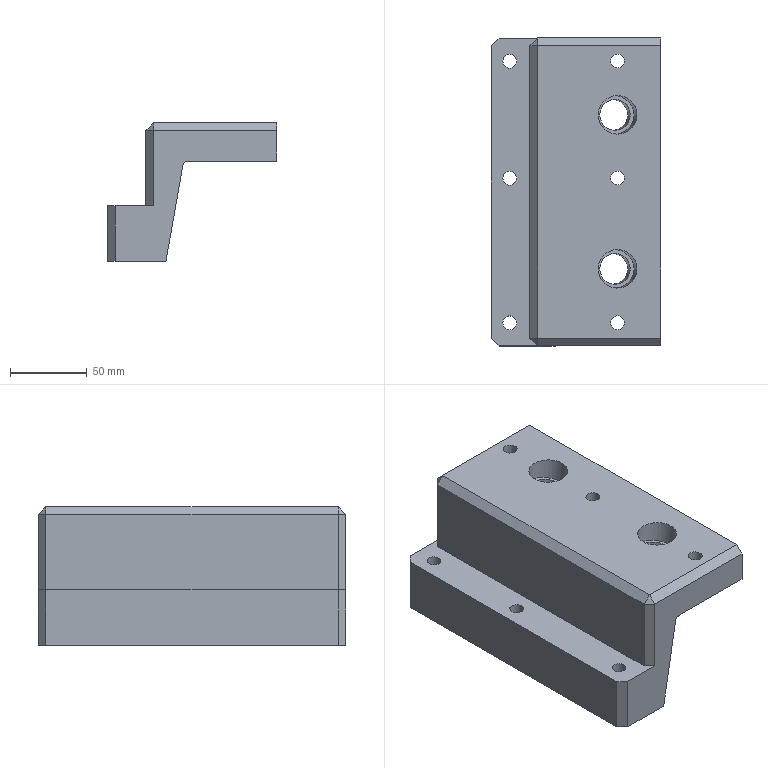Part | STEP file | P011002S003-012 | 1 solid | 44 faces | box 110 x 200 x 90 mm | volume 805824 mm3 | plane 27 | cylinder 17 | commonest cylinder face diameters 9 x6 14 x6 20 x2 25 x2 6 x1